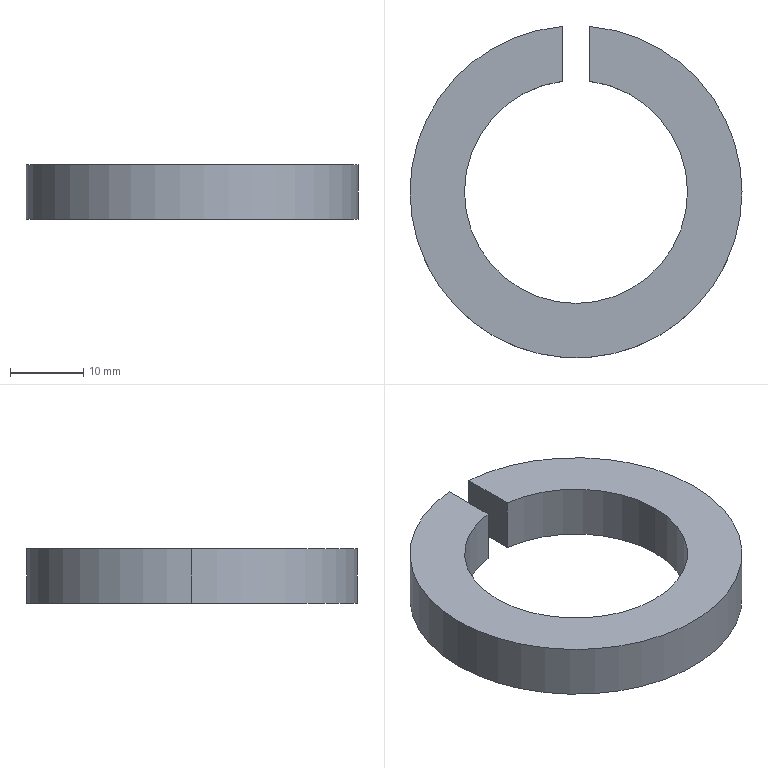Part | SolidWorks | features Extrusion 1 | 1 solid | 10 faces | box 45.424 x 45.346 x 7.5 mm | volume 6464 mm3 | cylinder 6 | plane 4 | commonest cylinder face diameters 30.5 x3 45.424 x3
STEP:
#1=CARTESIAN_POINT('',(15.25,0.,7.5));
#2=VERTEX_POINT('',#1);
#3=CARTESIAN_POINT('',(-15.25,0.,7.5));
#4=VERTEX_POINT('',#3);
#5=CARTESIAN_POINT('',(0.,0.,7.5));
#6=DIRECTION('',(0.,0.,-1.));
#7=DIRECTION('',(1.,0.,0.));
#8=AXIS2_PLACEMENT_3D('',#5,#6,#7);
#9=CIRCLE('',#8,15.25);
#10=EDGE_CURVE('',#2,#4,#9,.T.);
#11=ORIENTED_EDGE('',*,*,#10,.F.);
#12=CARTESIAN_POINT('',(15.25,0.,0.));
#13=VERTEX_POINT('',#12);
#14=CARTESIAN_POINT('',(15.25,0.,7.5));
#15=DIRECTION('',(0.,0.,-1.));
#16=VECTOR('',#15,1000.);
#17=LINE('',#14,#16);
#18=EDGE_CURVE('',#2,#13,#17,.T.);
#19=ORIENTED_EDGE('',*,*,#18,.T.);
#20=CARTESIAN_POINT('',(-15.25,0.,0.));
#21=VERTEX_POINT('',#20);
#22=CARTESIAN_POINT('',(0.,0.,0.));
#23=DIRECTION('',(0.,0.,-1.));
#24=DIRECTION('',(1.,0.,0.));
#25=AXIS2_PLACEMENT_3D('',#22,#23,#24);
#26=CIRCLE('',#25,15.25);
#27=EDGE_CURVE('',#13,#21,#26,.T.);
#28=ORIENTED_EDGE('',*,*,#27,.T.);
#29=CARTESIAN_POINT('',(-15.25,0.,7.5));
#30=DIRECTION('',(0.,0.,-1.));
#31=VECTOR('',#30,1000.);
#32=LINE('',#29,#31);
#33=EDGE_CURVE('',#4,#21,#32,.T.);
#34=ORIENTED_EDGE('',*,*,#33,.F.);
#35=EDGE_LOOP('',(#11,#19,#28,#34));
#36=FACE_OUTER_BOUND('',#35,.T.);
#37=CARTESIAN_POINT('',(0.,0.,7.5));
#38=DIRECTION('',(0.,0.,-1.));
#39=DIRECTION('',(-1.,0.,0.));
#40=AXIS2_PLACEMENT_3D('',#37,#38,#39);
#41=CYLINDRICAL_SURFACE('',#40,15.25);
#42=ADVANCED_FACE('',(#36),#41,.F.);
#43=CARTESIAN_POINT('',(-1.875,15.134,7.5));
#44=VERTEX_POINT('',#43);
#45=CARTESIAN_POINT('',(0.,0.,7.5));
#46=DIRECTION('',(0.,0.,-1.));
#47=DIRECTION('',(1.,0.,0.));
#48=AXIS2_PLACEMENT_3D('',#45,#46,#47);
#49=CIRCLE('',#48,15.25);
#50=EDGE_CURVE('',#4,#44,#49,.T.);
#51=ORIENTED_EDGE('',*,*,#50,.F.);
#52=ORIENTED_EDGE('',*,*,#33,.T.);
#53=CARTESIAN_POINT('',(-1.875,15.134,0.));
#54=VERTEX_POINT('',#53);
#55=CARTESIAN_POINT('',(0.,0.,0.));
#56=DIRECTION('',(0.,0.,-1.));
#57=DIRECTION('',(1.,0.,0.));
#58=AXIS2_PLACEMENT_3D('',#55,#56,#57);
#59=CIRCLE('',#58,15.25);
#60=EDGE_CURVE('',#21,#54,#59,.T.);
#61=ORIENTED_EDGE('',*,*,#60,.T.);
#62=CARTESIAN_POINT('',(-1.875,15.134,7.5));
#63=DIRECTION('',(0.,0.,-1.));
#64=VECTOR('',#63,1000.);
#65=LINE('',#62,#64);
#66=EDGE_CURVE('',#44,#54,#65,.T.);
#67=ORIENTED_EDGE('',*,*,#66,.F.);
#68=EDGE_LOOP('',(#51,#52,#61,#67));
#69=FACE_OUTER_BOUND('',#68,.T.);
#70=CARTESIAN_POINT('',(0.,0.,7.5));
#71=DIRECTION('',(0.,0.,-1.));
#72=DIRECTION('',(-1.,0.,0.));
#73=AXIS2_PLACEMENT_3D('',#70,#71,#72);
#74=CYLINDRICAL_SURFACE('',#73,15.25);
#75=ADVANCED_FACE('',(#69),#74,.F.);
#76=CARTESIAN_POINT('',(22.712,0.,7.5));
#77=VERTEX_POINT('',#76);
#78=CARTESIAN_POINT('',(1.875,22.634,7.5));
#79=VERTEX_POINT('',#78);
#80=CARTESIAN_POINT('',(0.,0.,7.5));
#81=DIRECTION('',(0.,0.,1.));
#82=DIRECTION('',(1.,0.,0.));
#83=AXIS2_PLACEMENT_3D('',#80,#81,#82);
#84=CIRCLE('',#83,22.712);
#85=EDGE_CURVE('',#77,#79,#84,.T.);
#86=ORIENTED_EDGE('',*,*,#85,.F.);
#87=CARTESIAN_POINT('',(22.712,0.,0.));
#88=VERTEX_POINT('',#87);
#89=CARTESIAN_POINT('',(22.712,0.,7.5));
#90=DIRECTION('',(0.,0.,-1.));
#91=VECTOR('',#90,1000.);
#92=LINE('',#89,#91);
#93=EDGE_CURVE('',#77,#88,#92,.T.);
#94=ORIENTED_EDGE('',*,*,#93,.T.);
#95=CARTESIAN_POINT('',(1.875,22.634,0.));
#96=VERTEX_POINT('',#95);
#97=CARTESIAN_POINT('',(0.,0.,0.));
#98=DIRECTION('',(0.,0.,1.));
#99=DIRECTION('',(1.,0.,0.));
#100=AXIS2_PLACEMENT_3D('',#97,#98,#99);
#101=CIRCLE('',#100,22.712);
#102=EDGE_CURVE('',#88,#96,#101,.T.);
#103=ORIENTED_EDGE('',*,*,#102,.T.);
#104=CARTESIAN_POINT('',(1.875,22.634,7.5));
#105=DIRECTION('',(0.,0.,-1.));
#106=VECTOR('',#105,1000.);
#107=LINE('',#104,#106);
#108=EDGE_CURVE('',#79,#96,#107,.T.);
#109=ORIENTED_EDGE('',*,*,#108,.F.);
#110=EDGE_LOOP('',(#86,#94,#103,#109));
#111=FACE_OUTER_BOUND('',#110,.T.);
#112=CARTESIAN_POINT('',(0.,0.,7.5));
#113=DIRECTION('',(0.,0.,-1.));
#114=DIRECTION('',(-1.,0.,0.));
#115=AXIS2_PLACEMENT_3D('',#112,#113,#114);
#116=CYLINDRICAL_SURFACE('',#115,22.712);
#117=ADVANCED_FACE('',(#111),#116,.T.);
#118=ORIENTED_EDGE('',*,*,#93,.F.);
#119=CARTESIAN_POINT('',(-22.712,0.,7.5));
#120=VERTEX_POINT('',#119);
#121=CARTESIAN_POINT('',(0.,0.,7.5));
#122=DIRECTION('',(0.,0.,1.));
#123=DIRECTION('',(1.,0.,0.));
#124=AXIS2_PLACEMENT_3D('',#121,#122,#123);
#125=CIRCLE('',#124,22.712);
#126=EDGE_CURVE('',#120,#77,#125,.T.);
#127=ORIENTED_EDGE('',*,*,#126,.F.);
#128=CARTESIAN_POINT('',(-22.712,0.,0.));
#129=VERTEX_POINT('',#128);
#130=CARTESIAN_POINT('',(-22.712,0.,7.5));
#131=DIRECTION('',(0.,0.,-1.));
#132=VECTOR('',#131,1000.);
#133=LINE('',#130,#132);
#134=EDGE_CURVE('',#120,#129,#133,.T.);
#135=ORIENTED_EDGE('',*,*,#134,.T.);
#136=CARTESIAN_POINT('',(0.,0.,0.));
#137=DIRECTION('',(0.,0.,1.));
#138=DIRECTION('',(1.,0.,0.));
#139=AXIS2_PLACEMENT_3D('',#136,#137,#138);
#140=CIRCLE('',#139,22.712);
#141=EDGE_CURVE('',#129,#88,#140,.T.);
#142=ORIENTED_EDGE('',*,*,#141,.T.);
#143=EDGE_LOOP('',(#118,#127,#135,#142));
#144=FACE_OUTER_BOUND('',#143,.T.);
#145=CARTESIAN_POINT('',(0.,0.,7.5));
#146=DIRECTION('',(0.,0.,-1.));
#147=DIRECTION('',(-1.,0.,0.));
#148=AXIS2_PLACEMENT_3D('',#145,#146,#147);
#149=CYLINDRICAL_SURFACE('',#148,22.712);
#150=ADVANCED_FACE('',(#144),#149,.T.);
#151=ORIENTED_EDGE('',*,*,#134,.F.);
#152=CARTESIAN_POINT('',(-1.875,22.634,7.5));
#153=VERTEX_POINT('',#152);
#154=CARTESIAN_POINT('',(0.,0.,7.5));
#155=DIRECTION('',(0.,0.,1.));
#156=DIRECTION('',(1.,0.,0.));
#157=AXIS2_PLACEMENT_3D('',#154,#155,#156);
#158=CIRCLE('',#157,22.712);
#159=EDGE_CURVE('',#153,#120,#158,.T.);
#160=ORIENTED_EDGE('',*,*,#159,.F.);
#161=CARTESIAN_POINT('',(-1.875,22.634,0.));
#162=VERTEX_POINT('',#161);
#163=CARTESIAN_POINT('',(-1.875,22.634,7.5));
#164=DIRECTION('',(0.,0.,-1.));
#165=VECTOR('',#164,1000.);
#166=LINE('',#163,#165);
#167=EDGE_CURVE('',#153,#162,#166,.T.);
#168=ORIENTED_EDGE('',*,*,#167,.T.);
#169=CARTESIAN_POINT('',(0.,0.,0.));
#170=DIRECTION('',(0.,0.,1.));
#171=DIRECTION('',(1.,0.,0.));
#172=AXIS2_PLACEMENT_3D('',#169,#170,#171);
#173=CIRCLE('',#172,22.712);
#174=EDGE_CURVE('',#162,#129,#173,.T.);
#175=ORIENTED_EDGE('',*,*,#174,.T.);
#176=EDGE_LOOP('',(#151,#160,#168,#175));
#177=FACE_OUTER_BOUND('',#176,.T.);
#178=CARTESIAN_POINT('',(0.,0.,7.5));
#179=DIRECTION('',(0.,0.,-1.));
#180=DIRECTION('',(-1.,0.,0.));
#181=AXIS2_PLACEMENT_3D('',#178,#179,#180);
#182=CYLINDRICAL_SURFACE('',#181,22.712);
#183=ADVANCED_FACE('',(#177),#182,.T.);
#184=CARTESIAN_POINT('',(1.875,15.134,0.));
#185=VERTEX_POINT('',#184);
#186=CARTESIAN_POINT('',(1.875,22.634,0.));
#187=DIRECTION('',(0.,-1.,0.));
#188=VECTOR('',#187,1000.);
#189=LINE('',#186,#188);
#190=EDGE_CURVE('',#96,#185,#189,.T.);
#191=ORIENTED_EDGE('',*,*,#190,.T.);
#192=CARTESIAN_POINT('',(1.875,15.134,7.5));
#193=VERTEX_POINT('',#192);
#194=CARTESIAN_POINT('',(1.875,15.134,7.5));
#195=DIRECTION('',(0.,0.,-1.));
#196=VECTOR('',#195,1000.);
#197=LINE('',#194,#196);
#198=EDGE_CURVE('',#193,#185,#197,.T.);
#199=ORIENTED_EDGE('',*,*,#198,.F.);
#200=CARTESIAN_POINT('',(1.875,22.634,7.5));
#201=DIRECTION('',(0.,-1.,0.));
#202=VECTOR('',#201,1000.);
#203=LINE('',#200,#202);
#204=EDGE_CURVE('',#79,#193,#203,.T.);
#205=ORIENTED_EDGE('',*,*,#204,.F.);
#206=ORIENTED_EDGE('',*,*,#108,.T.);
#207=EDGE_LOOP('',(#191,#199,#205,#206));
#208=FACE_OUTER_BOUND('',#207,.T.);
#209=CARTESIAN_POINT('',(1.875,22.634,7.5));
#210=DIRECTION('',(1.,0.,0.));
#211=DIRECTION('',(0.,1.,0.));
#212=AXIS2_PLACEMENT_3D('',#209,#210,#211);
#213=PLANE('',#212);
#214=ADVANCED_FACE('',(#208),#213,.F.);
#215=ORIENTED_EDGE('',*,*,#18,.F.);
#216=CARTESIAN_POINT('',(0.,0.,7.5));
#217=DIRECTION('',(0.,0.,-1.));
#218=DIRECTION('',(1.,0.,0.));
#219=AXIS2_PLACEMENT_3D('',#216,#217,#218);
#220=CIRCLE('',#219,15.25);
#221=EDGE_CURVE('',#193,#2,#220,.T.);
#222=ORIENTED_EDGE('',*,*,#221,.F.);
#223=ORIENTED_EDGE('',*,*,#198,.T.);
#224=CARTESIAN_POINT('',(0.,0.,0.));
#225=DIRECTION('',(0.,0.,-1.));
#226=DIRECTION('',(1.,0.,0.));
#227=AXIS2_PLACEMENT_3D('',#224,#225,#226);
#228=CIRCLE('',#227,15.25);
#229=EDGE_CURVE('',#185,#13,#228,.T.);
#230=ORIENTED_EDGE('',*,*,#229,.T.);
#231=EDGE_LOOP('',(#215,#222,#223,#230));
#232=FACE_OUTER_BOUND('',#231,.T.);
#233=CARTESIAN_POINT('',(0.,0.,7.5));
#234=DIRECTION('',(0.,0.,-1.));
#235=DIRECTION('',(-1.,0.,0.));
#236=AXIS2_PLACEMENT_3D('',#233,#234,#235);
#237=CYLINDRICAL_SURFACE('',#236,15.25);
#238=ADVANCED_FACE('',(#232),#237,.F.);
#239=CARTESIAN_POINT('',(-1.875,22.634,0.));
#240=DIRECTION('',(0.,1.,0.));
#241=VECTOR('',#240,1000.);
#242=LINE('',#239,#241);
#243=EDGE_CURVE('',#54,#162,#242,.T.);
#244=ORIENTED_EDGE('',*,*,#243,.T.);
#245=ORIENTED_EDGE('',*,*,#167,.F.);
#246=CARTESIAN_POINT('',(-1.875,22.634,7.5));
#247=DIRECTION('',(0.,1.,0.));
#248=VECTOR('',#247,1000.);
#249=LINE('',#246,#248);
#250=EDGE_CURVE('',#44,#153,#249,.T.);
#251=ORIENTED_EDGE('',*,*,#250,.F.);
#252=ORIENTED_EDGE('',*,*,#66,.T.);
#253=EDGE_LOOP('',(#244,#245,#251,#252));
#254=FACE_OUTER_BOUND('',#253,.T.);
#255=CARTESIAN_POINT('',(-1.875,22.634,7.5));
#256=DIRECTION('',(-1.,0.,0.));
#257=DIRECTION('',(0.,-1.,0.));
#258=AXIS2_PLACEMENT_3D('',#255,#256,#257);
#259=PLANE('',#258);
#260=ADVANCED_FACE('',(#254),#259,.F.);
#261=ORIENTED_EDGE('',*,*,#159,.T.);
#262=ORIENTED_EDGE('',*,*,#126,.T.);
#263=ORIENTED_EDGE('',*,*,#85,.T.);
#264=ORIENTED_EDGE('',*,*,#204,.T.);
#265=ORIENTED_EDGE('',*,*,#221,.T.);
#266=ORIENTED_EDGE('',*,*,#10,.T.);
#267=ORIENTED_EDGE('',*,*,#50,.T.);
#268=ORIENTED_EDGE('',*,*,#250,.T.);
#269=EDGE_LOOP('',(#261,#262,#263,#264,#265,#266,#267,#268));
#270=FACE_OUTER_BOUND('',#269,.T.);
#271=CARTESIAN_POINT('',(0.,0.,7.5));
#272=DIRECTION('',(0.,0.,1.));
#273=DIRECTION('',(1.,0.,0.));
#274=AXIS2_PLACEMENT_3D('',#271,#272,#273);
#275=PLANE('',#274);
#276=ADVANCED_FACE('',(#270),#275,.T.);
#277=ORIENTED_EDGE('',*,*,#174,.F.);
#278=ORIENTED_EDGE('',*,*,#243,.F.);
#279=ORIENTED_EDGE('',*,*,#60,.F.);
#280=ORIENTED_EDGE('',*,*,#27,.F.);
#281=ORIENTED_EDGE('',*,*,#229,.F.);
#282=ORIENTED_EDGE('',*,*,#190,.F.);
#283=ORIENTED_EDGE('',*,*,#102,.F.);
#284=ORIENTED_EDGE('',*,*,#141,.F.);
#285=EDGE_LOOP('',(#277,#278,#279,#280,#281,#282,#283,#284));
#286=FACE_OUTER_BOUND('',#285,.T.);
#287=CARTESIAN_POINT('',(0.,0.,0.));
#288=DIRECTION('',(0.,0.,1.));
#289=DIRECTION('',(1.,0.,0.));
#290=AXIS2_PLACEMENT_3D('',#287,#288,#289);
#291=PLANE('',#290);
#292=ADVANCED_FACE('',(#286),#291,.F.);
#293=CLOSED_SHELL('',(#42,#75,#117,#150,#183,#214,#238,#260,#276,#292));
#294=MANIFOLD_SOLID_BREP('',#293);
#295=CARTESIAN_POINT('',(0.,0.,0.));
#296=DIRECTION('',(0.,0.,1.));
#297=DIRECTION('',(1.,0.,0.));
#298=AXIS2_PLACEMENT_3D('',#295,#296,#297);
#299=(LENGTH_UNIT()NAMED_UNIT(*)SI_UNIT(.MILLI.,.METRE.));
#300=UNCERTAINTY_MEASURE_WITH_UNIT(LENGTH_MEASURE(0.00001),#299,'','');
#301=(NAMED_UNIT(*)PLANE_ANGLE_UNIT()SI_UNIT($,.RADIAN.));
#302=(NAMED_UNIT(*)SI_UNIT($,.STERADIAN.)SOLID_ANGLE_UNIT());
#303=(GEOMETRIC_REPRESENTATION_CONTEXT(3)GLOBAL_UNCERTAINTY_ASSIGNED_CONTEXT((#300))GLOBAL_UNIT_ASSIGNED_CONTEXT((#299,#301,#302))REPRESENTATION_CONTEXT('',''));
#304=ADVANCED_BREP_SHAPE_REPRESENTATION('',(#294,#298),#303);